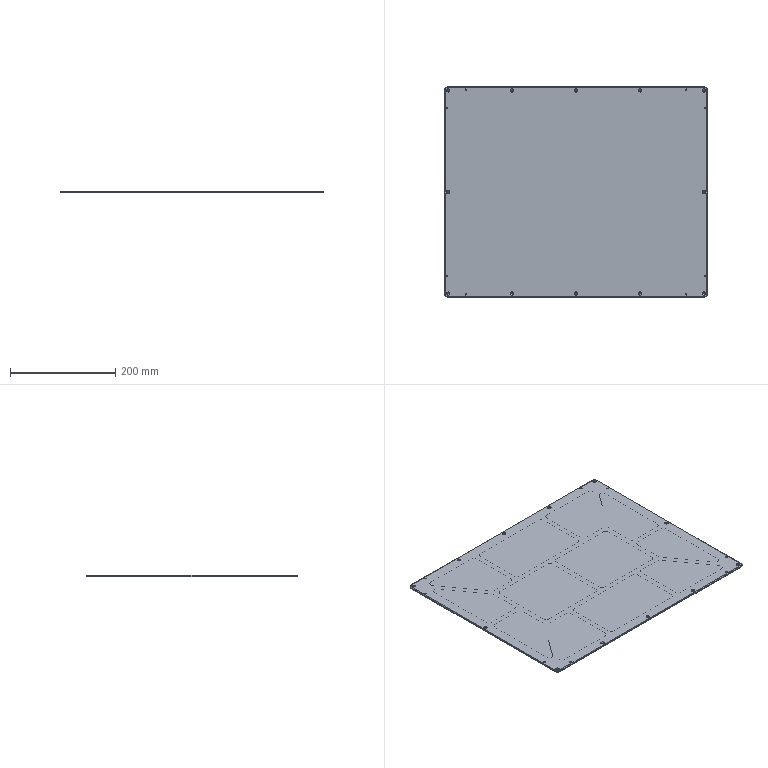NC program | Mastercam | posted with a generic post | part box 500 x 400 x 3 mm
Lines 215 to 2041 of 11256:
(8 BNOS |TOOL - 18|DIA. OFF. - 18|LEN. - 18|TOOL DIA. - 8.)
N508 T18 M6
N510 G0 G54 G90 X0. Y202.06 C0. B0. S7000 M3
N512 G43 H18 Z30.5
N514 Z19.999
N516 Z9.999
N518 G1 Z-.001 F600.
N520 X245. F4000.
N522 X245.315 Y202.053
N524 X245.958 Y201.995
N526 X246.613 Y201.873
N528 X247.272 Y201.685
N530 X247.761 Y201.498
N532 X248.243 Y201.271
N534 X248.711 Y201.006
N536 X249.161 Y200.703
N538 X249.59 Y200.364
N540 X249.992 Y199.992
N542 X250.364 Y199.59
N544 X250.703 Y199.161
N546 X251.006 Y198.711
N548 X251.271 Y198.243
N550 X251.498 Y197.761
N552 X251.685 Y197.272
N554 X251.788 Y196.943
N556 X251.942 Y196.285
N558 X252.032 Y195.634
N560 X252.06 Y195.
N562 Y-195.
N564 X252.053 Y-195.315
N566 X251.995 Y-195.958
N568 X251.873 Y-196.613
N570 X251.685 Y-197.272
N572 X251.498 Y-197.761
N574 X251.271 Y-198.243
N576 X251.006 Y-198.711
N578 X250.703 Y-199.161
N580 X250.364 Y-199.59
N582 X249.992 Y-199.992
N584 X249.59 Y-200.364
N586 X249.161 Y-200.703
N588 X248.711 Y-201.006
N590 X248.243 Y-201.271
N592 X247.761 Y-201.498
N594 X247.272 Y-201.685
N596 X246.943 Y-201.788
N598 X246.285 Y-201.942
N600 X245.634 Y-202.032
N602 X245. Y-202.06
N604 X-245.
N606 X-245.315 Y-202.053
N608 X-245.958 Y-201.995
N610 X-246.613 Y-201.873
N612 X-247.272 Y-201.685
N614 X-247.761 Y-201.498
N616 X-248.243 Y-201.271
N618 X-248.711 Y-201.006
N620 X-249.161 Y-200.703
N622 X-249.59 Y-200.364
N624 X-249.992 Y-199.992
N626 X-250.364 Y-199.59
N628 X-250.703 Y-199.161
N630 X-251.006 Y-198.711
N632 X-251.271 Y-198.243
N634 X-251.498 Y-197.761
N636 X-251.685 Y-197.272
N638 X-251.788 Y-196.943
N640 X-251.942 Y-196.285
N642 X-252.032 Y-195.634
N644 X-252.06 Y-195.
N646 Y195.
N648 X-252.053 Y195.315
N650 X-251.995 Y195.958
N652 X-251.873 Y196.613
N654 X-251.685 Y197.272
N656 X-251.498 Y197.761
N658 X-251.271 Y198.243
N660 X-251.006 Y198.711
N662 X-250.703 Y199.161
N664 X-250.364 Y199.59
N666 X-249.992 Y199.992
N668 X-249.59 Y200.364
N670 X-249.161 Y200.703
N672 X-248.711 Y201.006
N674 X-248.243 Y201.271
N676 X-247.761 Y201.498
N678 X-247.272 Y201.685
N680 X-246.943 Y201.788
N682 X-246.285 Y201.942
N684 X-245.634 Y202.032
N686 X-245. Y202.06
N688 X0.
N690 X245.336 Y202.079 Z-.002
N692 X245.979 Y202.018
N694 X246.634 Y201.896
N696 X247.293 Y201.706
N698 X247.782 Y201.518
N700 X248.264 Y201.291
N702 X248.732 Y201.025
N704 X249.182 Y200.722
N706 X249.611 Y200.383
N708 X250.013 Y200.01
N710 X250.386 Y199.608
N712 X250.724 Y199.179
N714 X251.028 Y198.728
N716 X251.293 Y198.26
N718 X251.521 Y197.779
N720 X251.708 Y197.289
N722 X251.811 Y196.96
N724 X251.967 Y196.302
N726 X252.057 Y195.651
N728 X252.088 Y195.017
N730 X252.13 Y-195.043 Z-.004
N732 X252.12 Y-195.358
N734 X252.058 Y-196.002
N736 X251.935 Y-196.657
N738 X251.744 Y-197.316
N740 X251.556 Y-197.806
N742 X251.328 Y-198.287
N744 X251.062 Y-198.756
N746 X250.758 Y-199.207
N748 X250.419 Y-199.636
N750 X250.047 Y-200.039
N752 X249.644 Y-200.412
N754 X249.216 Y-200.752
N756 X248.765 Y-201.056
N758 X248.297 Y-201.323
N760 X247.816 Y-201.552
N762 X247.327 Y-201.741
N764 X246.998 Y-201.846
N766 X246.34 Y-202.004
N768 X245.689 Y-202.096
N770 X245.055 Y-202.13
N772 X-245.096 Y-202.182 Z-.008
N774 X-245.411 Y-202.171
N776 X-246.055 Y-202.104
N778 X-246.711 Y-201.979 Z-.009
N780 X-247.369 Y-201.783
N782 X-247.858 Y-201.593
N784 X-248.339 Y-201.363
N786 X-248.807 Y-201.094
N788 X-249.257 Y-200.789
N790 X-249.686 Y-200.449
N792 X-250.089 Y-200.075
N794 X-250.462 Y-199.672
N796 X-250.801 Y-199.242
N798 X-251.105 Y-198.791
N800 X-251.373 Y-198.322
N802 X-251.601 Y-197.841
N804 X-251.791 Y-197.35
N806 X-251.896 Y-197.022
N808 X-252.056 Y-196.363
N810 X-252.149 Y-195.712
N812 X-252.184 Y-195.077
N814 X-252.226 Y195.103 Z-.013
N816 X-252.213 Y195.419
N818 X-252.145 Y196.063
N820 X-252.022 Y196.719
N822 X-251.827 Y197.378
N824 X-251.637 Y197.868
N826 X-251.407 Y198.349
N828 X-251.14 Y198.818
N830 X-250.835 Y199.27
N832 X-250.496 Y199.7
N834 X-250.123 Y200.104
N836 X-249.72 Y200.478
N838 X-249.291 Y200.819
N840 X-248.84 Y201.125
N842 X-248.373 Y201.394
N844 X-247.892 Y201.626
N846 X-247.403 Y201.818
N848 X-247.074 Y201.926
N850 X-246.417 Y202.089
N852 X-245.765 Y202.186
N854 X-245.13 Y202.226
N856 X0. Y202.259 Z-.017
N858 X245.021 Y202.287 Z-.021
N860 X245.674 Y202.255
N862 X246.342 Y202.162
N864 X246.68 Y202.09
N866 X247.019 Y202.001
N868 X247.357 Y201.895
N870 X247.861 Y201.702
N872 X248.355 Y201.468
N874 X248.837 Y201.195
N876 X249.3 Y200.883
N878 X249.741 Y200.534
N880 X250.154 Y200.151
N882 X250.537 Y199.737
N884 X250.885 Y199.296
N886 X251.197 Y198.833
N888 X251.47 Y198.352
N890 X251.704 Y197.857
N892 X251.897 Y197.353
N894 X252.003 Y197.015
N896 X252.092 Y196.676
N898 X252.163 Y196.338
N900 X252.257 Y195.67
N902 X252.288 Y195.017
N904 X252.331 Y-195.044 Z-.028
N906 X252.298 Y-195.697
N908 X252.203 Y-196.366
N910 X252.131 Y-196.704
N912 X252.041 Y-197.043
N914 X251.934 Y-197.381
N916 X251.74 Y-197.884
N918 X251.505 Y-198.379
N920 X251.231 Y-198.861 Z-.027
N922 X250.919 Y-199.324
N924 X250.57 Y-199.765 Z-.028
N926 X250.188 Y-200.18
N928 X249.774 Y-200.563
N930 X249.333 Y-200.912 Z-.027
N932 X248.87 Y-201.225
N934 X248.389 Y-201.5
N936 X247.895 Y-201.735 Z-.028
N938 X247.392 Y-201.93
N940 X247.054 Y-202.038
N942 X246.715 Y-202.128
N944 X246.377 Y-202.201
N946 X245.709 Y-202.297
N948 X245.056 Y-202.332
N950 X-245.098 Y-202.387 Z-.038
N952 X-245.752 Y-202.349
N954 X-246.42 Y-202.249
N956 X-246.758 Y-202.175
N958 X-247.097 Y-202.083
N960 X-247.435 Y-201.974
N962 X-247.938 Y-201.777
N964 X-248.432 Y-201.541
N966 X-248.913 Y-201.264
N968 X-249.376 Y-200.95
N970 X-249.816 Y-200.6
N972 X-250.23 Y-200.216
N974 X-250.613 Y-199.801
N976 X-250.962 Y-199.359
N978 X-251.275 Y-198.896
N980 X-251.549 Y-198.414
N982 X-251.785 Y-197.919
N984 X-251.98 Y-197.416
N986 X-252.089 Y-197.078
N988 X-252.18 Y-196.739
N990 X-252.254 Y-196.401
N992 X-252.352 Y-195.732
N994 X-252.388 Y-195.079
N996 X-252.431 Y195.106 Z-.047
N998 X-252.393 Y195.759
N1000 X-252.293 Y196.429
N1002 X-252.219 Y196.767
N1004 X-252.127 Y197.105
N1006 X-252.017 Y197.444
N1008 X-251.821 Y197.947
N1010 X-251.585 Y198.442
N1012 X-251.309 Y198.924
N1014 X-250.996 Y199.387
N1016 X-250.646 Y199.829
N1018 X-250.263 Y200.244
N1020 X-249.849 Y200.628
N1022 X-249.409 Y200.979
N1024 X-248.946 Y201.294
N1026 X-248.466 Y201.571
N1028 X-247.972 Y201.809
N1030 X-247.469 Y202.007
N1032 X-247.132 Y202.12
N1034 X-246.456 Y202.288
N1036 X-245.787 Y202.391
N1038 X-245.133 Y202.431
N1040 X0. Y202.462 Z-.054
N1042 X245.188 Y202.486 Z-.06
N1044 X245.523 Y202.47
N1046 X245.863 Y202.438
N1048 X246.207 Y202.39
N1050 X246.553 Y202.325
N1052 X247.075 Y202.197 Z-.061
N1054 X247.596 Y202.026
N1056 X248.111 Y201.814
N1058 X248.616 Y201.56
N1060 X249.105 Y201.265
N1062 X249.574 Y200.932
N1064 X250.018 Y200.561
N1066 X250.433 Y200.157
N1068 X250.815 Y199.722
N1070 X251.161 Y199.26
N1072 X251.469 Y198.777
N1074 X251.736 Y198.277
N1076 X251.962 Y197.765
N1078 X252.146 Y197.245
N1080 X252.29 Y196.723
N1082 X252.363 Y196.376
N1084 X252.419 Y196.03
N1086 X252.459 Y195.688
N1088 X252.483 Y195.35
N1090 X252.491 Y195.017
N1092 X252.531 Y-195.211 Z-.072
N1094 X252.514 Y-195.546
N1096 X252.481 Y-195.887
N1098 X252.432 Y-196.231
N1100 X252.366 Y-196.577
N1102 X252.237 Y-197.099 Z-.073
N1104 X252.065 Y-197.62
N1106 X251.852 Y-198.136
N1108 X251.598 Y-198.64
N1110 X251.303 Y-199.13
N1112 X250.97 Y-199.6
N1114 X250.599 Y-200.044
N1116 X250.195 Y-200.46
N1118 X249.759 Y-200.843
N1120 X249.298 Y-201.19
N1122 X248.815 Y-201.498
N1124 X248.316 Y-201.767
N1126 X247.803 Y-201.995
N1128 X247.284 Y-202.181
N1130 X246.762 Y-202.326
N1132 X246.415 Y-202.402
N1134 X246.07 Y-202.459
N1136 X245.727 Y-202.501
N1138 X245.223 Y-202.531
N1140 X-245.099 Y-202.591 Z-.089
N1142 X-245.601 Y-202.566
N1144 X-245.942 Y-202.531
N1146 X-246.286 Y-202.48
N1148 X-246.632 Y-202.412
N1150 X-247.153 Y-202.279
N1152 X-247.674 Y-202.104
N1154 X-248.189 Y-201.889
N1156 X-248.693 Y-201.632
N1158 X-249.182 Y-201.336
N1160 X-249.651 Y-201. Z-.09
N1162 X-250.096 Y-200.629
N1164 X-250.511 Y-200.223
N1166 X-250.894 Y-199.787
N1168 X-251.24 Y-199.325
N1170 X-251.549 Y-198.841
N1172 X-251.818 Y-198.341
N1174 X-252.046 Y-197.828
N1176 X-252.232 Y-197.309
N1178 X-252.378 Y-196.786 Z-.089
N1180 X-252.454 Y-196.439 Z-.09
N1182 X-252.513 Y-196.093
N1184 X-252.555 Y-195.751
N1186 X-252.592 Y-195.079
N1188 X-252.636 Y195.106 Z-.104
N1190 X-252.624 Y195.44
N1192 X-252.596 Y195.778
N1194 X-252.553 Y196.121
N1196 X-252.494 Y196.466
N1198 X-252.418 Y196.814
N1200 X-252.323 Y197.162
N1202 X-252.149 Y197.683
N1204 X-251.934 Y198.199
N1206 X-251.678 Y198.704
N1208 X-251.382 Y199.194
N1210 X-251.048 Y199.664
N1212 X-250.677 Y200.11
N1214 X-250.272 Y200.526
N1216 X-249.836 Y200.91
N1218 X-249.375 Y201.259
N1220 X-248.893 Y201.57
N1222 X-248.393 Y201.841
N1224 X-247.881 Y202.072
N1226 X-247.362 Y202.261
N1228 X-246.841 Y202.41
N1230 X-246.494 Y202.489
N1232 X-246.148 Y202.55
N1234 X-245.806 Y202.594
N1236 X-245.134 Y202.636
N1238 X0. Y202.666 Z-.114
N1240 X245.192 Y202.689 Z-.123
N1242 X245.537 Y202.673
N1244 X245.886 Y202.64
N1246 X246.239 Y202.591
N1248 X246.595 Y202.524
N1250 X247.131 Y202.393 Z-.124
N1252 X247.666 Y202.217
N1254 X248.195 Y201.999
N1256 X248.713 Y201.738
N1258 X249.216 Y201.436
N1260 X249.698 Y201.093
N1262 X250.154 Y200.712
N1264 X250.581 Y200.297
N1266 X250.973 Y199.85
N1268 X251.328 Y199.376
N1270 X251.644 Y198.879
N1272 X251.919 Y198.366
N1274 X252.151 Y197.839
N1276 X252.34 Y197.306
N1278 X252.488 Y196.769
N1280 X252.563 Y196.412
N1282 X252.621 Y196.058
N1284 X252.662 Y195.706
N1286 X252.686 Y195.359 Z-.125
N1288 X252.695 Y195.017
N1290 X252.734 Y-195.215 Z-.141
N1292 X252.716 Y-195.56
N1294 X252.683 Y-195.909
N1296 X252.633 Y-196.262
N1298 X252.565 Y-196.618 Z-.14
N1300 X252.432 Y-197.155 Z-.141
N1302 X252.256 Y-197.69
N1304 X252.037 Y-198.219
N1306 X251.775 Y-198.738
N1308 X251.472 Y-199.24
N1310 X251.129 Y-199.722
N1312 X250.749 Y-200.179
N1314 X250.333 Y-200.606
N1316 X249.887 Y-201.
N1318 X249.413 Y-201.356
N1320 X248.917 Y-201.673
N1322 X248.404 Y-201.949
N1324 X247.878 Y-202.183
N1326 X247.344 Y-202.374
N1328 X246.808 Y-202.524
N1330 X246.451 Y-202.602
N1332 X246.097 Y-202.66
N1334 X245.745 Y-202.703 Z-.142
N1336 X245.398 Y-202.729
N1338 X245.056 Y-202.739
N1340 X-245.098 Y-202.793 Z-.164
N1342 X-245.44 Y-202.782
N1344 X-245.788 Y-202.754
N1346 X-246.139 Y-202.71
N1348 X-246.494 Y-202.649
N1350 X-246.851 Y-202.57
N1352 X-247.209 Y-202.474
N1354 X-247.743 Y-202.295
N1356 X-248.272 Y-202.073
N1358 X-248.79 Y-201.809
N1360 X-249.292 Y-201.504
N1362 X-249.773 Y-201.16
N1364 X-250.23 Y-200.777
N1366 X-250.656 Y-200.361
N1368 X-251.049 Y-199.913
N1370 X-251.405 Y-199.438
N1372 X-251.722 Y-198.942
N1374 X-251.998 Y-198.428
N1376 X-252.232 Y-197.902
N1378 X-252.424 Y-197.368
N1380 X-252.574 Y-196.832
N1382 X-252.653 Y-196.475
N1384 X-252.713 Y-196.12
N1386 X-252.757 Y-195.768 Z-.165
N1388 X-252.784 Y-195.421
N1390 X-252.795 Y-195.078
N1392 X-252.837 Y195.105 Z-.184
N1394 X-252.825 Y195.448
N1396 X-252.798 Y195.795
N1398 X-252.754 Y196.147
N1400 X-252.693 Y196.502
N1402 X-252.614 Y196.859
N1404 X-252.517 Y197.217 Z-.183
N1406 X-252.338 Y197.752
N1408 X-252.116 Y198.281
N1410 X-251.853 Y198.8
N1412 X-251.549 Y199.303
N1414 X-251.205 Y199.785
N1416 X-250.824 Y200.242
N1418 X-250.408 Y200.67
N1420 X-249.961 Y201.065
N1422 X-249.488 Y201.423
N1424 X-248.992 Y201.742
N1426 X-248.48 Y202.021
N1428 X-247.954 Y202.257
N1430 X-247.421 Y202.452
N1432 X-246.885 Y202.606
N1434 X-246.529 Y202.688 Z-.184
N1436 X-245.998 Y202.772 Z-.183
N1438 X-245.649 Y202.81
N1440 X-245.133 Y202.838 Z-.184
N1442 X0. Y202.868 Z-.198
N1444 X245.196 Y202.89 Z-.21
N1446 X245.549 Y202.873
N1448 X245.908 Y202.84
N1450 X246.27 Y202.789
N1452 X246.818 Y202.682 Z-.211
N1454 X247.369 Y202.53
N1456 X247.917 Y202.336
N1458 X248.457 Y202.097
N1460 X248.984 Y201.815
N1462 X249.493 Y201.491
N1464 X249.979 Y201.126
N1466 X250.438 Y200.723
N1468 X250.865 Y200.286
N1470 X251.255 Y199.817
N1472 X251.606 Y199.322
N1474 X251.917 Y198.806
N1476 X252.184 Y198.274
N1478 X252.408 Y197.731
N1480 X252.587 Y197.182
N1482 X252.724 Y196.631
N1484 X252.82 Y196.085
N1486 X252.862 Y195.724
N1488 X252.887 Y195.368
N1490 X252.895 Y195.017 Z-.212
N1492 X252.933 Y-195.218 Z-.233
N1494 X252.915 Y-195.572
N1496 X252.881 Y-195.931 Z-.232
N1498 X252.83 Y-196.293
N1500 X252.721 Y-196.841 Z-.233
N1502 X252.569 Y-197.392 Z-.234
N1504 X252.374 Y-197.94
N1506 X252.135 Y-198.48
N1508 X251.852 Y-199.008
N1510 X251.528 Y-199.517
N1512 X251.163 Y-200.004
N1514 X250.76 Y-200.464
N1516 X250.322 Y-200.891
N1518 X249.853 Y-201.282
N1520 X249.359 Y-201.634
N1522 X248.843 Y-201.946
N1524 X248.312 Y-202.215
N1526 X247.769 Y-202.44
N1528 X247.219 Y-202.621
N1530 X246.669 Y-202.76 Z-.233
N1532 X246.122 Y-202.858
N1534 X245.761 Y-202.902 Z-.234
N1536 X245.405 Y-202.928
N1538 X245.054 Y-202.938
N1540 X-245.095 Y-202.991 Z-.263
N1542 X-245.446 Y-202.979
N1544 X-245.803 Y-202.951
N1546 X-246.164 Y-202.906
N1548 X-246.528 Y-202.844
N1550 X-246.894 Y-202.763
N1552 X-247.444 Y-202.608
N1554 X-247.992 Y-202.41
N1556 X-248.531 Y-202.169
N1558 X-249.058 Y-201.884
N1560 X-249.567 Y-201.558
N1562 X-250.054 Y-201.192
N1564 X-250.513 Y-200.787 Z-.264
N1566 X-250.939 Y-200.349
N1568 X-251.33 Y-199.88
N1570 X-251.683 Y-199.384
N1572 X-251.994 Y-198.868
N1574 X-252.263 Y-198.336
N1576 X-252.489 Y-197.792 Z-.263
N1578 X-252.671 Y-197.243
N1580 X-252.81 Y-196.692
N1582 X-252.909 Y-196.145
N1584 X-252.954 Y-195.784
N1586 X-252.981 Y-195.427 Z-.264
N1588 X-252.992 Y-195.076
N1590 X-253.033 Y195.102 Z-.288
N1592 X-253.021 Y195.453
N1594 X-252.993 Y195.81
N1596 X-252.948 Y196.171
N1598 X-252.886 Y196.536
N1600 X-252.805 Y196.902
N1602 X-252.65 Y197.453
N1604 X-252.453 Y198.001
N1606 X-252.212 Y198.541
N1608 X-251.928 Y199.069
N1610 X-251.602 Y199.579
N1612 X-251.237 Y200.066 Z-.289
N1614 X-250.833 Y200.526
N1616 X-250.395 Y200.954
N1618 X-249.927 Y201.347 Z-.288
N1620 X-249.433 Y201.701
N1622 X-248.917 Y202.014
N1624 X-248.386 Y202.286
N1626 X-247.843 Y202.514
N1628 X-247.294 Y202.699
N1630 X-246.744 Y202.841 Z-.287
N1632 X-246.197 Y202.943
N1634 X-245.837 Y202.99 Z-.288
N1636 X-245.48 Y203.02
N1638 X-245.128 Y203.033
N1640 X0. Y203.062 Z-.305
N1642 X245.199 Y203.083 Z-.32
N1644 X245.561 Y203.066
N1646 X245.929 Y203.032
N1648 X246.3 Y202.98
N1650 X246.862 Y202.87 Z-.321
N1652 X247.426 Y202.715
N1654 X247.987 Y202.516 Z-.322
N1656 X248.541 Y202.271
N1658 X249.081 Y201.982 Z-.321
N1660 X249.603 Y201.65 Z-.322
N1662 X250.101 Y201.276
N1664 X250.571 Y200.863
N1666 X251.008 Y200.415
N1668 X251.408 Y199.935
N1670 X251.768 Y199.428
N1672 X252.086 Y198.899
N1674 X252.36 Y198.354
N1676 X252.589 Y197.797
N1678 X252.773 Y197.234
N1680 X252.913 Y196.671
N1682 X253.011 Y196.11
N1684 X253.054 Y195.74
N1686 X253.079 Y195.375
N1688 X253.088 Y195.016
N1690 X253.124 Y-195.22 Z-.348
N1692 X253.106 Y-195.583
N1694 X253.071 Y-195.95
N1696 X253.019 Y-196.322
N1698 X252.907 Y-196.884 Z-.349
N1700 X252.751 Y-197.448
N1702 X252.551 Y-198.009
N1704 X252.307 Y-198.563
N1706 X252.017 Y-199.104
N1708 X251.685 Y-199.626
N1710 X251.311 Y-200.125
N1712 X250.898 Y-200.595 Z-.35
N1714 X250.449 Y-201.033 Z-.349
N1716 X249.969 Y-201.433
N1718 X249.463 Y-201.795
N1720 X248.934 Y-202.114
N1722 X248.389 Y-202.389
N1724 X247.833 Y-202.62
N1726 X247.27 Y-202.805
N1728 X246.706 Y-202.948
N1730 X246.146 Y-203.048
N1732 X245.776 Y-203.092
N1734 X245.411 Y-203.119
N1736 X245.051 Y-203.129
N1738 X-245.09 Y-203.179 Z-.385
N1740 X-245.45 Y-203.167
N1742 X-245.815 Y-203.139
N1744 X-246.185 Y-203.093
N1746 X-246.558 Y-203.03
N1748 X-246.933 Y-202.947 Z-.384
N1750 X-247.497 Y-202.789 Z-.385
N1752 X-248.058 Y-202.586
N1754 X-248.611 Y-202.339
N1756 X-249.151 Y-202.048
N1758 X-249.673 Y-201.714
N1760 X-250.171 Y-201.338
N1762 X-250.641 Y-200.924 Z-.386
N1764 X-251.079 Y-200.475
N1766 X-251.479 Y-199.994
N1768 X-251.84 Y-199.486 Z-.385
N1770 X-252.159 Y-198.957
N1772 X-252.435 Y-198.412
N1774 X-252.666 Y-197.855
N1776 X-252.852 Y-197.292
N1778 X-252.995 Y-196.728
N1780 X-253.096 Y-196.167
N1782 X-253.141 Y-195.797
N1784 X-253.169 Y-195.432
N1786 X-253.18 Y-195.072
N1788 X-253.219 Y195.096 Z-.415
N1790 X-253.193 Y195.639 Z-.414
N1792 X-253.156 Y196.007 Z-.413
N1794 X-253.101 Y196.379
N1796 X-252.986 Y196.941 Z-.414
N1798 X-252.828 Y197.505 Z-.415
N1800 X-252.626 Y198.067
N1802 X-252.38 Y198.62
N1804 X-252.089 Y199.161
N1806 X-251.755 Y199.683
N1808 X-251.381 Y200.183 Z-.416
N1810 X-250.967 Y200.654
N1812 X-250.519 Y201.092 Z-.415
N1814 X-250.039 Y201.495
N1816 X-249.532 Y201.857
N1818 X-249.004 Y202.178
N1820 X-248.459 Y202.456
N1822 X-247.903 Y202.689
N1824 X-247.341 Y202.879 Z-.414
N1826 X-246.777 Y203.024
N1828 X-246.217 Y203.128
N1830 X-245.847 Y203.176 Z-.415
N1832 X-245.122 Y203.219
N1834 X0. Y203.245 Z-.435
N1836 X245.202 Y203.265 Z-.453
N1838 X245.572 Y203.248
N1840 X245.948 Y203.213
N1842 X246.328 Y203.16
N1844 X246.902 Y203.047 Z-.454
N1846 X247.479 Y202.888
N1848 X248.053 Y202.685
N1850 X248.619 Y202.435
N1852 X249.172 Y202.139
N1854 X249.705 Y201.8
N1856 X250.215 Y201.418 Z-.455
N1858 X250.696 Y200.995
N1860 X251.143 Y200.537
N1862 X251.552 Y200.045 Z-.454
N1864 X251.92 Y199.527 Z-.455
N1866 X252.245 Y198.986
N1868 X252.525 Y198.429
N1870 X252.76 Y197.859
N1872 X252.948 Y197.284
N1874 X253.091 Y196.707
N1876 X253.192 Y196.134
N1878 X253.235 Y195.756
N1880 X253.261 Y195.382
N1882 X253.27 Y195.015
N1884 X253.303 Y-195.221 Z-.485
N1886 X253.285 Y-195.592
N1888 X253.249 Y-195.968
N1890 X253.195 Y-196.348
N1892 X253.081 Y-196.922 Z-.486
N1894 X252.922 Y-197.499
N1896 X252.717 Y-198.074
N1898 X252.467 Y-198.64
N1900 X252.171 Y-199.192
N1902 X251.831 Y-199.726
N1904 X251.449 Y-200.237 Z-.487
N1906 X251.027 Y-200.718
N1908 X250.568 Y-201.166
N1910 X250.077 Y-201.575
N1912 X249.559 Y-201.945
N1914 X249.019 Y-202.271
N1916 X248.462 Y-202.553
N1918 X247.892 Y-202.788
N1920 X247.317 Y-202.978
N1922 X246.74 Y-203.123
N1924 X246.167 Y-203.225
N1926 X245.789 Y-203.27
N1928 X245.415 Y-203.298
N1930 X245.047 Y-203.308
N1932 X-245.083 Y-203.354 Z-.528
N1934 X-245.451 Y-203.342
N1936 X-245.825 Y-203.313
N1938 X-246.203 Y-203.267
N1940 X-246.585 Y-203.202 Z-.527
N1942 X-246.968 Y-203.117
N1944 X-247.545 Y-202.956
N1946 X-248.119 Y-202.749
N1948 X-248.684 Y-202.497
N1950 X-249.236 Y-202.199
N1952 X-249.77 Y-201.857
N1954 X-250.28 Y-201.475 Z-.529
N1956 X-250.76 Y-201.051 Z-.528
N1958 X-251.208 Y-200.591 Z-.529
N1960 X-251.617 Y-200.1 Z-.528
N1962 X-251.987 Y-199.581 Z-.529
N1964 X-252.312 Y-199.04 Z-.528
N1966 X-252.595 Y-198.482 Z-.529
N1968 X-252.831 Y-197.913
N1970 X-253.021 Y-197.337
N1972 X-253.167 Y-196.76
N1974 X-253.27 Y-196.187
N1976 X-253.316 Y-195.808
N1978 X-253.344 Y-195.435
N1980 X-253.354 Y-195.066
N1982 X-253.385 Y195.273 Z-.562
N1984 X-253.365 Y195.644
N1986 X-253.327 Y196.02 Z-.561
N1988 X-253.271 Y196.4
N1990 X-253.153 Y196.975
N1992 X-252.991 Y197.552
N1994 X-252.785 Y198.126
N1996 X-252.533 Y198.692
N1998 X-252.236 Y199.245
N2000 X-251.894 Y199.779
N2002 X-251.513 Y200.291 Z-.563
N2004 X-251.09 Y200.772 Z-.562
N2006 X-250.632 Y201.22 Z-.563
N2008 X-250.141 Y201.631 Z-.562
N2010 X-249.623 Y202.002 Z-.563
N2012 X-249.083 Y202.33
N2014 X-248.526 Y202.614
N2016 X-247.957 Y202.852
N2018 X-247.382 Y203.045
N2020 X-246.806 Y203.194
N2022 X-246.232 Y203.3
N2024 X-245.854 Y203.348
N2026 X-245.481 Y203.378
N2028 X-245.112 Y203.39
N2030 X0. Y203.414 Z-.586
N2032 X245.226 Y203.431 Z-.606
N2034 X245.623 Y203.411
N2036 X246.19 Y203.351 Z-.607
N2038 X246.766 Y203.249 Z-.608
N2040 X247.345 Y203.103
N2042 X247.922 Y202.913
N2044 X248.426 Y202.709
N2046 X248.974 Y202.441
N2048 X249.506 Y202.131
N2050 X250.019 Y201.78
N2052 X250.348 Y201.524
N2054 X250.664 Y201.252
N2056 X250.966 Y200.964
N2058 X251.294 Y200.617
N2060 X251.571 Y200.29
N2062 X251.831 Y199.95
N2064 X252.072 Y199.599
N2066 X252.295 Y199.237
N2068 X252.497 Y198.868
N2070 X252.68 Y198.492
N2072 X252.915 Y197.919
N2074 X253.105 Y197.342
N2076 X253.25 Y196.763
N2078 X253.352 Y196.187
N2080 X253.397 Y195.808
N2082 X253.425 Y195.432
N2084 X253.436 Y195.013
N2086 X253.47 Y-195.033 Z-.644
N2088 X253.458 Y-195.453
N2090 X253.429 Y-195.828
N2092 X253.383 Y-196.208
N2094 X253.28 Y-196.784
N2096 X253.134 Y-197.363
N2098 X252.943 Y-197.941
N2100 X252.738 Y-198.445
N2102 X252.47 Y-198.992
N2104 X252.16 Y-199.525
N2106 X251.809 Y-200.038
N2108 X251.553 Y-200.367
N2110 X251.281 Y-200.684 Z-.645
N2112 X250.993 Y-200.987
N2114 X250.646 Y-201.315
N2116 X250.319 Y-201.593
N2118 X249.979 Y-201.853
N2120 X249.628 Y-202.095 Z-.644
N2122 X249.267 Y-202.318
N2124 X248.897 Y-202.521 Z-.645
N2126 X248.521 Y-202.704
N2128 X247.949 Y-202.941 Z-.644
N2130 X247.371 Y-203.132
N2132 X246.793 Y-203.279
N2134 X246.217 Y-203.383
N2136 X245.837 Y-203.429
N2138 X245.462 Y-203.458
N2140 X245.042 Y-203.471 Z-.645
N2142 X-245.074 Y-203.511 Z-.691
N2144 X-245.494 Y-203.497 Z-.69
N2146 X-246.059 Y-203.444 Z-.689
N2148 X-246.249 Y-203.419 Z-.69
N2150 X-246.825 Y-203.314
N2152 X-247.404 Y-203.165 Z-.691
N2154 X-247.981 Y-202.973
N2156 X-248.485 Y-202.766
N2158 X-249.032 Y-202.496 Z-.69
N2160 X-249.564 Y-202.184 Z-.691
N2162 X-250.077 Y-201.832
N2164 X-250.405 Y-201.576
N2166 X-250.722 Y-201.303
N2168 X-251.025 Y-201.014 Z-.692
N2170 X-251.352 Y-200.667 Z-.691
N2172 X-251.63 Y-200.339
N2174 X-251.89 Y-199.998
N2176 X-252.132 Y-199.647
N2178 X-252.355 Y-199.286 Z-.692
N2180 X-252.558 Y-198.916
N2182 X-252.742 Y-198.54
N2184 X-252.978 Y-197.967 Z-.691
N2186 X-253.17 Y-197.389
N2188 X-253.317 Y-196.81
N2190 X-253.422 Y-196.235
N2192 X-253.485 Y-195.667 Z-.69
N2194 X-253.512 Y-195.059 Z-.691
N2196 X-253.544 Y195.08 Z-.729
N2198 X-253.529 Y195.5
N2200 X-253.476 Y196.065 Z-.728
N2202 X-253.451 Y196.255 Z-.729
N2204 X-253.345 Y196.831
N2206 X-253.197 Y197.41
N2208 X-253.005 Y197.988
N2210 X-252.799 Y198.492
N2212 X-252.529 Y199.039
N2214 X-252.218 Y199.572
N2216 X-251.866 Y200.085
N2218 X-251.61 Y200.414 Z-.73
N2220 X-251.338 Y200.731
N2222 X-251.05 Y201.035
N2224 X-250.703 Y201.363
N2226 X-250.376 Y201.642
N2228 X-250.036 Y201.903
N2230 X-249.685 Y202.146
N2232 X-249.324 Y202.37
N2234 X-248.955 Y202.574
N2236 X-248.579 Y202.759
N2238 X-248.007 Y202.998 Z-.729
N2240 X-247.43 Y203.192
N2242 X-246.851 Y203.342
N2244 X-246.276 Y203.449
N2246 X-245.708 Y203.514 Z-.728
N2248 X-245.101 Y203.544 Z-.73
N2250 X0. Y203.565 Z-.755
N2252 X245.205 Y203.58 Z-.777
N2254 X245.59 Y203.563
N2256 X245.98 Y203.527
N2258 X246.375 Y203.472
N2260 X246.772 Y203.398
N2262 X247.171 Y203.303
N2264 X247.571 Y203.189
N2266 X247.969 Y203.053
N2268 X248.364 Y202.896
N2270 X248.755 Y202.718
N2272 X249.139 Y202.519
N2274 X249.516 Y202.299
N2276 X249.883 Y202.058
N2278 X250.239 Y201.798
N2280 X250.582 Y201.52
N2282 X250.911 Y201.223 Z-.778
N2284 X251.225 Y200.909
N2286 X251.521 Y200.58
N2288 X251.8 Y200.237
N2290 X252.06 Y199.881 Z-.777
N2292 X252.3 Y199.514 Z-.778
N2294 X252.52 Y199.137
N2296 X252.719 Y198.753
N2298 X252.897 Y198.362
N2300 X253.054 Y197.967
N2302 X253.19 Y197.568
N2304 X253.305 Y197.169
N2306 X253.399 Y196.77
N2308 X253.473 Y196.372
N2310 X253.527 Y195.978
N2312 X253.563 Y195.587
N2314 X253.581 Y195.202
N2316 X253.61 Y-195.22 Z-.817
N2318 X253.591 Y-195.605
N2320 X253.555 Y-195.995
N2322 X253.5 Y-196.39
N2324 X253.425 Y-196.788
N2326 X253.33 Y-197.187
N2328 X253.215 Y-197.587
N2330 X253.079 Y-197.985
N2332 X252.922 Y-198.38
N2334 X252.743 Y-198.771
N2336 X252.544 Y-199.156
N2338 X252.324 Y-199.532
N2340 X252.083 Y-199.9
N2342 X251.823 Y-200.256
N2344 X251.544 Y-200.599
N2346 X251.248 Y-200.929 Z-.818
N2348 X250.934 Y-201.243
N2350 X250.605 Y-201.54 Z-.817
N2352 X250.262 Y-201.819
N2354 X249.906 Y-202.079
N2356 X249.539 Y-202.32
N2358 X249.162 Y-202.54
N2360 X248.778 Y-202.74 Z-.818
N2362 X248.387 Y-202.919
N2364 X247.992 Y-203.077
N2366 X247.594 Y-203.213
N2368 X247.195 Y-203.329
N2370 X246.795 Y-203.424 Z-.817
N2372 X246.398 Y-203.499 Z-.818
N2374 X246.003 Y-203.555
N2376 X245.613 Y-203.591
N2378 X245.227 Y-203.61
N2380 X-245.064 Y-203.649 Z-.869
N2382 X-245.446 Y-203.638
N2384 X-245.834 Y-203.609
N2386 X-246.227 Y-203.562
N2388 X-246.624 Y-203.496
N2390 X-247.022 Y-203.41
N2392 X-247.422 Y-203.304
N2394 X-247.821 Y-203.177
N2396 X-248.218 Y-203.029 Z-.87
N2398 X-248.611 Y-202.86
N2400 X-248.999 Y-202.67
N2402 X-249.379 Y-202.459
N2404 X-249.751 Y-202.228
N2406 X-250.113 Y-201.977
N2408 X-250.463 Y-201.707
N2410 X-250.8 Y-201.418
N2412 X-251.121 Y-201.112
N2414 X-251.427 Y-200.79
N2416 X-251.715 Y-200.453
N2418 X-251.985 Y-200.103
N2420 X-252.235 Y-199.741
N2422 X-252.466 Y-199.368
N2424 X-252.676 Y-198.987
N2426 X-252.866 Y-198.599
N2428 X-253.034 Y-198.206
N2430 X-253.182 Y-197.809
N2432 X-253.308 Y-197.41
N2434 X-253.413 Y-197.01
N2436 X-253.499 Y-196.611
N2438 X-253.564 Y-196.214
N2440 X-253.611 Y-195.822
N2442 X-253.639 Y-195.433
N2444 X-253.65 Y-195.051
N2446 X-253.673 Y195.26 Z-.91
N2448 X-253.653 Y195.645
N2450 X-253.615 Y196.036
N2452 X-253.558 Y196.431
N2454 X-253.482 Y196.828
N2456 X-253.386 Y197.228
N2458 X-253.269 Y197.627
N2460 X-253.132 Y198.025
N2462 X-252.974 Y198.421
N2464 X-252.795 Y198.812
N2466 X-252.595 Y199.196
N2468 X-252.374 Y199.573
N2470 X-252.133 Y199.94
N2472 X-251.873 Y200.297
N2474 X-251.594 Y200.641
N2476 X-251.297 Y200.97
N2478 X-250.983 Y201.284
N2480 X-250.654 Y201.582
N2482 X-250.311 Y201.862
N2484 X-249.955 Y202.123
N2486 X-249.588 Y202.365
N2488 X-249.212 Y202.586
N2490 X-248.827 Y202.787
N2492 X-248.437 Y202.967
N2494 X-248.042 Y203.126
N2496 X-247.644 Y203.264
N2498 X-247.245 Y203.381
N2500 X-246.846 Y203.478
N2502 X-246.448 Y203.555
N2504 X-246.054 Y203.613
N2506 X-245.663 Y203.652
N2508 X-245.278 Y203.673
N2510 X0. Y203.695 Z-.938
N2512 X245.205 Y203.708 Z-.963
N2514 X245.596 Y203.69
N2516 X245.992 Y203.653
N2518 X246.393 Y203.598
N2520 X246.797 Y203.523
N2522 X247.202 Y203.427
N2524 X247.607 Y203.31
N2526 X248.012 Y203.173
N2528 X248.413 Y203.014
N2530 X248.809 Y202.833
N2532 X249.2 Y202.631
N2534 X249.582 Y202.407
N2536 X249.955 Y202.163
N2538 X250.316 Y201.899
N2540 X250.664 Y201.616
N2542 X250.999 Y201.315
N2544 X251.317 Y200.997
N2546 X251.618 Y200.663
N2548 X251.901 Y200.314
N2550 X252.165 Y199.953
N2552 X252.409 Y199.58
N2554 X252.632 Y199.198
N2556 X252.834 Y198.807
N2558 X253.015 Y198.411
N2560 X253.174 Y198.01
N2562 X253.311 Y197.605
N2564 X253.428 Y197.2
N2566 X253.523 Y196.794
N2568 X253.599 Y196.391
N2570 X253.654 Y195.99
N2572 X253.69 Y195.594
N2574 X253.708 Y195.203 Z-.964
N2576 X253.732 Y-195.218 Z-1.005
N2578 X253.714 Y-195.609
N2580 X253.677 Y-196.005
N2582 X253.621 Y-196.406
N2584 X253.545 Y-196.809
N2586 X253.449 Y-197.215
N2588 X253.333 Y-197.621
N2590 X253.195 Y-198.025
N2592 X253.035 Y-198.426
N2594 X252.854 Y-198.823
N2596 X252.652 Y-199.213
N2598 X252.428 Y-199.596
N2600 X252.184 Y-199.969
N2602 X251.92 Y-200.33
N2604 X251.637 Y-200.679
N2606 X251.336 Y-201.013
N2608 X251.018 Y-201.332
N2610 X250.684 Y-201.633
N2612 X250.335 Y-201.917
N2614 X249.974 Y-202.181
N2616 X249.601 Y-202.425
N2618 X249.219 Y-202.649
N2620 X248.828 Y-202.852
N2622 X248.432 Y-203.033 Z-1.006
N2624 X248.031 Y-203.193
N2626 X247.627 Y-203.331
N2628 X247.221 Y-203.448
N2630 X246.816 Y-203.544
N2632 X246.412 Y-203.62
N2634 X246.011 Y-203.677
N2636 X245.615 Y-203.714
N2638 X245.224 Y-203.733
N2640 X-245.053 Y-203.765 Z-1.06
N2642 X-245.441 Y-203.754
N2644 X-245.835 Y-203.726
N2646 X-246.234 Y-203.678
N2648 X-246.636 Y-203.611
N2650 X-247.041 Y-203.525
N2652 X-247.446 Y-203.417
N2654 X-247.852 Y-203.289
N2656 X-248.255 Y-203.139
N2658 X-248.654 Y-202.968
N2660 X-249.047 Y-202.775
N2662 X-249.434 Y-202.562
N2664 X-249.812 Y-202.327
N2666 X-250.179 Y-202.072 Z-1.061
N2668 X-250.534 Y-201.798
N2670 X-250.876 Y-201.505
N2672 X-251.202 Y-201.195
N2674 X-251.512 Y-200.868
N2676 X-251.805 Y-200.526
N2678 X-252.079 Y-200.17
N2680 X-252.333 Y-199.803
N2682 X-252.567 Y-199.425
N2684 X-252.78 Y-199.038
N2686 X-252.973 Y-198.644
N2688 X-253.143 Y-198.245
N2690 X-253.292 Y-197.842
N2692 X-253.42 Y-197.436
N2694 X-253.527 Y-197.03
N2696 X-253.614 Y-196.626
N2698 X-253.68 Y-196.223
N2700 X-253.727 Y-195.824
N2702 X-253.755 Y-195.43
N2704 X-253.766 Y-195.042
N2706 X-253.784 Y195.251 Z-1.103
N2708 X-253.764 Y195.642
N2710 X-253.726 Y196.038
N2712 X-253.669 Y196.439
N2714 X-253.592 Y196.843
N2716 X-253.495 Y197.248
N2718 X-253.377 Y197.654
N2720 X-253.238 Y198.058
N2722 X-253.078 Y198.46
N2724 X-252.896 Y198.856
N2726 X-252.693 Y199.247
N2728 X-252.469 Y199.629
N2730 X-252.225 Y200.002
N2732 X-251.961 Y200.364
N2734 X-251.678 Y200.713
N2736 X-251.376 Y201.047
N2738 X-251.058 Y201.366
N2740 X-250.724 Y201.668
N2742 X-250.375 Y201.952
N2744 X-250.014 Y202.217
N2746 X-249.642 Y202.462
N2748 X-249.259 Y202.686
N2750 X-248.869 Y202.89
N2752 X-248.473 Y203.072
N2754 X-248.072 Y203.233
N2756 X-247.668 Y203.373
N2758 X-247.263 Y203.491
N2760 X-246.857 Y203.589
N2762 X-246.454 Y203.667
N2764 X-246.053 Y203.724
N2766 X-245.657 Y203.763 Z-1.104
N2768 X-245.266 Y203.784
N2770 X0. Y203.802 Z-1.132
N2772 X245.205 Y203.812 Z-1.158
N2774 X245.601 Y203.794
N2776 X246.002 Y203.757
N2778 X246.408 Y203.701
N2780 X246.816 Y203.625
N2782 X247.226 Y203.528
N2784 X247.637 Y203.411
N2786 X248.046 Y203.271
N2788 X248.452 Y203.11
N2790 X248.854 Y202.927
N2792 X249.249 Y202.723
N2794 X249.636 Y202.497
N2796 X250.013 Y202.25
N2798 X250.379 Y201.983
N2800 X250.732 Y201.696
N2802 X251.07 Y201.391 Z-1.159
N2804 X251.392 Y201.069
N2806 X251.697 Y200.731
N2808 X251.984 Y200.378
N2810 X252.251 Y200.012
N2812 X252.498 Y199.635
N2814 X252.724 Y199.248
N2816 X252.928 Y198.852
N2818 X253.111 Y198.451
N2820 X253.272 Y198.045
N2822 X253.411 Y197.635
N2824 X253.529 Y197.225
N2826 X253.626 Y196.815
N2828 X253.702 Y196.406
N2830 X253.758 Y196.
N2832 X253.794 Y195.599
N2834 X253.812 Y195.204
N2836 X253.832 Y-195.215 Z-1.203
N2838 X253.813 Y-195.611
N2840 X253.776 Y-196.012
N2842 X253.72 Y-196.418 Z-1.202
N2844 X253.643 Y-196.826
N2846 X253.546 Y-197.237
N2848 X253.428 Y-197.647 Z-1.203
N2850 X253.289 Y-198.057
N2852 X253.127 Y-198.463
N2854 X252.944 Y-198.865
N2856 X252.739 Y-199.26
N2858 X252.513 Y-199.647
N2860 X252.266 Y-200.024
N2862 X251.999 Y-200.39
N2864 X251.712 Y-200.743
N2866 X251.408 Y-201.082
N2868 X251.085 Y-201.404
N2870 X250.747 Y-201.709
N2872 X250.394 Y-201.996
N2874 X250.028 Y-202.264
N2876 X249.651 Y-202.511
N2878 X249.264 Y-202.737
N2880 X248.869 Y-202.942
N2882 X248.467 Y-203.125
N2884 X248.061 Y-203.287
N2886 X247.652 Y-203.427
N2888 X247.241 Y-203.545
N2890 X246.831 Y-203.642
N2892 X246.422 Y-203.719
N2894 X246.017 Y-203.776
N2896 X245.616 Y-203.813
N2898 X245.22 Y-203.832
N2900 X-245.041 Y-203.858 Z-1.259
N2902 X-245.434 Y-203.847
N2904 X-245.833 Y-203.819
N2906 X-246.236 Y-203.771
N2908 X-246.644 Y-203.704
N2910 X-247.054 Y-203.616
N2912 X-247.464 Y-203.508
N2914 X-247.874 Y-203.379 Z-1.26
N2916 X-248.282 Y-203.227
N2918 X-248.686 Y-203.054
N2920 X-249.085 Y-202.86
N2922 X-249.476 Y-202.644
N2924 X-249.859 Y-202.406
N2926 X-250.231 Y-202.149
N2928 X-250.59 Y-201.871
N2930 X-250.936 Y-201.575
N2932 X-251.267 Y-201.261
N2934 X-251.58 Y-200.93
N2936 X-251.877 Y-200.584
N2938 X-252.154 Y-200.224
N2940 X-252.411 Y-199.852
N2942 X-252.648 Y-199.469
N2944 X-252.864 Y-199.078
N2946 X-253.058 Y-198.679
N2948 X-253.231 Y-198.275
N2950 X-253.381 Y-197.867
N2952 X-253.511 Y-197.456
N2954 X-253.619 Y-197.046
N2956 X-253.706 Y-196.636
N2958 X-253.773 Y-196.228
N2960 X-253.82 Y-195.825
N2962 X-253.848 Y-195.426
N2964 X-253.858 Y-195.033
N2966 X-253.872 Y195.241 Z-1.304
N2968 X-253.852 Y195.637
N2970 X-253.814 Y196.038
N2972 X-253.757 Y196.444
N2974 X-253.679 Y196.852
N2976 X-253.582 Y197.263
N2978 X-253.463 Y197.673
N2980 X-253.322 Y198.083
N2982 X-253.16 Y198.489
N2984 X-252.977 Y198.89
N2986 X-252.772 Y199.286
N2988 X-252.545 Y199.673
N2990 X-252.298 Y200.05
N2992 X-252.03 Y200.416
N2994 X-251.744 Y200.77
N2996 X-251.439 Y201.108
N2998 X-251.116 Y201.431
N3000 X-250.778 Y201.736
N3002 X-250.425 Y202.024
N3004 X-250.06 Y202.291
N3006 X-249.683 Y202.539
N3008 X-249.296 Y202.766
N3010 X-248.901 Y202.972
N3012 X-248.499 Y203.156
N3014 X-248.093 Y203.319
N3016 X-247.684 Y203.459
N3018 X-247.274 Y203.579
N3020 X-246.864 Y203.677
N3022 X-246.455 Y203.755
N3024 X-246.049 Y203.813
N3026 X-245.648 Y203.851
N3028 X-245.252 Y203.872 Z-1.305
N3030 X0. Y203.886 Z-1.334
N3032 X245.205 Y203.893 Z-1.36
N3034 X245.604 Y203.874
N3036 X246.009 Y203.838
N3038 X246.418 Y203.781
N3040 X246.831 Y203.704
N3042 X247.245 Y203.607
N3044 X247.66 Y203.488
N3046 X248.073 Y203.347
N3048 X248.483 Y203.185
N3050 X248.888 Y203. Z-1.361
N3052 X249.287 Y202.794 Z-1.36
N3054 X249.678 Y202.566
N3056 X250.059 Y202.317
N3058 X250.428 Y202.047
N3060 X250.784 Y201.758 Z-1.361
N3062 X251.125 Y201.45
N3064 X251.451 Y201.125
N3066 X251.759 Y200.783
N3068 X252.048 Y200.427
N3070 X252.317 Y200.058
N3072 X252.566 Y199.677
N3074 X252.794 Y199.286
N3076 X253.001 Y198.887
N3078 X253.185 Y198.482
N3080 X253.348 Y198.071
N3082 X253.489 Y197.658
N3084 X253.607 Y197.244
N3086 X253.705 Y196.83
N3088 X253.782 Y196.417
N3090 X253.838 Y196.008
N3092 X253.875 Y195.603
N3094 X253.893 Y195.203
N3096 X253.907 Y-195.211 Z-1.405
N3098 X253.889 Y-195.611
N3100 X253.851 Y-196.016
N3102 X253.795 Y-196.426
N3104 X253.718 Y-196.838
N3106 X253.62 Y-197.253
N3108 X253.501 Y-197.667
N3110 X253.36 Y-198.08
N3112 X253.197 Y-198.49
N3114 X253.013 Y-198.896
N3116 X252.806 Y-199.295
N3118 X252.578 Y-199.686
N3120 X252.329 Y-200.067
N3122 X252.059 Y-200.436
N3124 X251.77 Y-200.792
N3126 X251.462 Y-201.134 Z-1.406
N3128 X251.137 Y-201.459
N3130 X250.795 Y-201.767
N3132 X250.439 Y-202.057
N3134 X250.07 Y-202.327
N3136 X249.689 Y-202.576
N3138 X249.298 Y-202.804
N3140 X248.899 Y-203.011
N3142 X248.494 Y-203.196
N3144 X248.084 Y-203.359
N3146 X247.67 Y-203.5
N3148 X247.256 Y-203.619
N3150 X246.842 Y-203.717
N3152 X246.429 Y-203.794
N3154 X246.02 Y-203.851
N3156 X245.615 Y-203.889
N3158 X245.215 Y-203.907
N3160 X-245.03 Y-203.926 Z-1.463
N3162 X-245.426 Y-203.916
N3164 X-245.829 Y-203.888
N3166 X-246.236 Y-203.84
N3168 X-246.647 Y-203.773
N3170 X-247.061 Y-203.685
N3172 X-247.476 Y-203.576
N3174 X-247.89 Y-203.446
N3176 X-248.302 Y-203.294
N3178 X-248.709 Y-203.119
N3180 X-249.112 Y-202.923
N3182 X-249.507 Y-202.705
N3184 X-249.893 Y-202.466
N3186 X-250.268 Y-202.206
N3188 X-250.631 Y-201.926
N3190 X-250.981 Y-201.627
N3192 X-251.314 Y-201.31
N3194 X-251.631 Y-200.976
N3196 X-251.93 Y-200.627
N3198 X-252.21 Y-200.264
N3200 X-252.469 Y-199.888
N3202 X-252.708 Y-199.502
N3204 X-252.926 Y-199.107
N3206 X-253.122 Y-198.704 Z-1.464
N3208 X-253.296 Y-198.296
N3210 X-253.448 Y-197.884
N3212 X-253.578 Y-197.47 Z-1.463
N3214 X-253.687 Y-197.055
N3216 X-253.774 Y-196.641
N3218 X-253.842 Y-196.23 Z-1.464
N3220 X-253.889 Y-195.823
N3222 X-253.917 Y-195.42
N3224 X-253.927 Y-195.024
N3226 X-253.936 Y195.23 Z-1.508
N3228 X-253.916 Y195.63
N3230 X-253.878 Y196.035
N3232 X-253.821 Y196.444
N3234 X-253.744 Y196.857
N3236 X-253.645 Y197.271
N3238 X-253.526 Y197.686
N3240 X-253.384 Y198.099
N3242 X-253.221 Y198.509
N3244 X-253.036 Y198.914
N3246 X-252.829 Y199.313
N3248 X-252.601 Y199.704
N3250 X-252.351 Y200.085
N3252 X-252.081 Y200.455
N3254 X-251.792 Y200.811
N3256 X-251.484 Y201.153
N3258 X-251.159 Y201.478
N3260 X-250.817 Y201.787
N3262 X-250.461 Y202.076
N3264 X-250.092 Y202.346
N3266 X-249.711 Y202.596
N3268 X-249.321 Y202.825
N3270 X-248.922 Y203.032
N3272 X-248.516 Y203.218
N3274 X-248.107 Y203.381
N3276 X-247.694 Y203.523
N3278 X-247.279 Y203.643
N3280 X-246.865 Y203.742
N3282 X-246.452 Y203.82
N3284 X-246.043 Y203.878 Z-1.509
N3286 X-245.638 Y203.916
N3288 X-245.238 Y203.936
N3290 X0. Y203.946 Z-1.538
N3292 X245.203 Y203.95 Z-1.565
N3294 X245.606 Y203.932
N3296 X246.013 Y203.895
N3298 X246.425 Y203.838
N3300 X246.841 Y203.761
N3302 X247.258 Y203.663
N3304 X247.675 Y203.543
N3306 X248.091 Y203.402
N3308 X248.51 Y203.235
N3310 X248.93 Y203.043
N3312 X249.342 Y202.828
N3314 X249.746 Y202.59
N3316 X250.129 Y202.337
N3318 X250.489 Y202.072
N3320 X250.836 Y201.788
N3322 X251.169 Y201.487
N3324 X251.492 Y201.164
N3326 X251.802 Y200.82
N3328 X252.093 Y200.462
N3330 X252.364 Y200.09
N3332 X252.615 Y199.706
N3334 X252.845 Y199.313
N3336 X253.053 Y198.911
N3338 X253.238 Y198.503
N3340 X253.402 Y198.09
N3342 X253.543 Y197.674
N3344 X253.663 Y197.257
N3346 X253.761 Y196.84
N3348 X253.838 Y196.425
N3350 X253.895 Y196.013
N3352 X253.932 Y195.605
N3354 X253.95 Y195.203 Z-1.566
N3356 X253.959 Y-195.208 Z-1.61
N3358 X253.941 Y-195.61
N3360 X253.904 Y-196.018
N3362 X253.847 Y-196.43
N3364 X253.769 Y-196.845
N3366 X253.671 Y-197.263
N3368 X253.551 Y-197.68
N3370 X253.41 Y-198.096
N3372 X253.244 Y-198.515
N3374 X253.052 Y-198.935
N3376 X252.836 Y-199.348
N3378 X252.598 Y-199.752
N3380 X252.345 Y-200.134
N3382 X252.08 Y-200.494
N3384 X251.796 Y-200.842
N3386 X251.495 Y-201.175
N3388 X251.172 Y-201.498
N3390 X250.828 Y-201.808
N3392 X250.469 Y-202.099
N3394 X250.097 Y-202.371
N3396 X249.714 Y-202.622
N3398 X249.321 Y-202.851
N3400 X248.919 Y-203.059
N3402 X248.511 Y-203.245
N3404 X248.098 Y-203.409
N3406 X247.682 Y-203.551
N3408 X247.265 Y-203.671
N3410 X246.848 Y-203.769
N3412 X246.432 Y-203.846
N3414 X246.02 Y-203.903
N3416 X245.612 Y-203.941
N3418 X245.21 Y-203.959
N3420 X-245.018 Y-203.972 Z-1.667
N3422 X-245.417 Y-203.962
N3424 X-245.823 Y-203.934
N3426 X-246.233 Y-203.887
N3428 X-246.647 Y-203.82
N3430 X-247.063 Y-203.732
N3432 X-247.481 Y-203.622
N3434 X-247.898 Y-203.491
N3436 X-248.312 Y-203.338
N3438 X-248.735 Y-203.158
N3440 X-249.152 Y-202.954
N3442 X-249.56 Y-202.727
N3444 X-249.959 Y-202.477
N3446 X-250.325 Y-202.221
N3448 X-250.679 Y-201.946
N3450 X-251.02 Y-201.653
N3452 X-251.346 Y-201.343
N3454 X-251.665 Y-201.007
N3456 X-251.965 Y-200.655
N3458 X-252.247 Y-200.29
N3460 X-252.508 Y-199.912
N3462 X-252.749 Y-199.523
N3464 X-252.968 Y-199.125
N3466 X-253.165 Y-198.72
N3468 X-253.34 Y-198.309
N3470 X-253.493 Y-197.894
N3472 X-253.623 Y-197.477
N3474 X-253.732 Y-197.06
N3476 X-253.82 Y-196.643
N3478 X-253.888 Y-196.229
N3480 X-253.935 Y-195.819
N3482 X-253.963 Y-195.414
N3484 X-253.972 Y-195.015 Z-1.668
N3486 X-253.976 Y195.219 Z-1.712
N3488 X-253.958 Y195.621
N3490 X-253.92 Y196.029
N3492 X-253.863 Y196.442
N3494 X-253.785 Y196.857
N3496 X-253.686 Y197.274
N3498 X-253.566 Y197.691
N3500 X-253.424 Y198.107
N3502 X-253.26 Y198.52
N3504 X-253.074 Y198.928
N3506 X-252.866 Y199.33
N3508 X-252.636 Y199.723
N3510 X-252.385 Y200.107
N3512 X-252.114 Y200.479
N3514 X-251.823 Y200.838
N3516 X-251.513 Y201.181
N3518 X-251.19 Y201.505
N3520 X-250.857 Y201.806
N3522 X-250.509 Y202.09
N3524 X-250.15 Y202.356
N3526 X-249.767 Y202.609
N3528 X-249.363 Y202.848
N3530 X-248.95 Y203.063
N3532 X-248.531 Y203.256
N3534 X-248.112 Y203.423
N3536 X-247.696 Y203.565
N3538 X-247.279 Y203.685
N3540 X-246.862 Y203.784
N3542 X-246.447 Y203.862
N3544 X-246.034 Y203.919
N3546 X-245.627 Y203.957
N3548 X-245.224 Y203.976
N3550 X0. Y203.983 Z-1.741
N3552 X245.202 Y203.984 Z-1.768
N3554 X245.606 Y203.966
N3556 X246.015 Y203.929
N3558 X246.429 Y203.872
N3560 X246.846 Y203.795
N3562 X247.265 Y203.696
N3564 X247.684 Y203.576
N3566 X248.102 Y203.434
N3568 X248.523 Y203.267
N3570 X248.946 Y203.074
N3572 X249.362 Y202.857
N3574 X249.769 Y202.617
N3576 X250.153 Y202.362
N3578 X250.513 Y202.097
N3580 X250.86 Y201.813
N3582 X251.193 Y201.511
N3584 X251.517 Y201.188
N3586 X251.828 Y200.843
N3588 X252.12 Y200.483
N3590 X252.393 Y200.109
N3592 X252.645 Y199.724
N3594 X252.875 Y199.329
N3596 X253.084 Y198.926
N3598 X253.27 Y198.516
N3600 X253.434 Y198.101
N3602 X253.576 Y197.684
N3604 X253.697 Y197.265
N3606 X253.795 Y196.846
N3608 X253.872 Y196.429
N3610 X253.929 Y196.015
N3612 X253.966 Y195.605
N3614 X253.984 Y195.202
N3616 X253.989 Y-195.204 Z-1.812
N3618 X253.971 Y-195.608
N3620 X253.933 Y-196.017
N3622 X253.876 Y-196.431
N3624 X253.799 Y-196.848
N3626 X253.701 Y-197.267
N3628 X253.58 Y-197.686
N3630 X253.438 Y-198.104
N3632 X253.271 Y-198.525
N3634 X253.078 Y-198.948
N3636 X252.861 Y-199.364
N3638 X252.621 Y-199.771
N3640 X252.366 Y-200.155
N3642 X252.101 Y-200.515
N3644 X251.817 Y-200.863
N3646 X251.515 Y-201.196
N3648 X251.191 Y-201.52
N3650 X250.846 Y-201.831
N3652 X250.486 Y-202.123
N3654 X250.113 Y-202.396
N3656 X249.728 Y-202.648
N3658 X249.333 Y-202.878
N3660 X248.929 Y-203.087
N3662 X248.519 Y-203.274
N3664 X248.105 Y-203.438
N3666 X247.687 Y-203.58
N3668 X247.268 Y-203.7
N3670 X246.849 Y-203.799
N3672 X246.432 Y-203.876
N3674 X246.018 Y-203.933
N3676 X245.609 Y-203.971
N3678 X245.205 Y-203.989 Z-1.813
N3680 X-245.008 Y-203.996 Z-1.867
N3682 X-245.408 Y-203.986
N3684 X-245.815 Y-203.959
N3686 X-246.227 Y-203.911
N3688 X-246.643 Y-203.844
N3690 X-247.061 Y-203.756
N3692 X-247.48 Y-203.647
N3694 X-247.899 Y-203.516
N3696 X-248.315 Y-203.362
N3698 X-248.741 Y-203.181
N3700 X-249.161 Y-202.975
N3702 X-249.573 Y-202.746 Z-1.868
N3704 X-249.776 Y-202.623 Z-1.867
N3706 X-250.159 Y-202.369
N3708 X-250.519 Y-202.103
N3710 X-250.867 Y-201.819
N3712 X-251.2 Y-201.517
N3714 X-251.524 Y-201.194
N3716 X-251.835 Y-200.848 Z-1.868
N3718 X-252.127 Y-200.488
N3720 X-252.4 Y-200.115
N3722 X-252.652 Y-199.73
N3724 X-252.882 Y-199.335
N3726 X-253.091 Y-198.931
N3728 X-253.278 Y-198.521
N3730 X-253.442 Y-198.107
N3732 X-253.584 Y-197.689
N3734 X-253.705 Y-197.27
N3736 X-253.803 Y-196.851
N3738 X-253.881 Y-196.434
N3740 X-253.938 Y-196.02
N3742 X-253.975 Y-195.611
N3744 X-253.993 Y-195.207
N3746 X-253.996 Y195.209 Z-1.911
N3748 X-253.977 Y195.613
N3750 X-253.94 Y196.022
N3752 X-253.883 Y196.436
N3754 X-253.805 Y196.853
N3756 X-253.707 Y197.272
N3758 X-253.586 Y197.691
N3760 X-253.444 Y198.109
N3762 X-253.28 Y198.523
N3764 X-253.093 Y198.933 Z-1.912
N3766 X-252.884 Y199.336
N3768 X-252.654 Y199.731
N3770 X-252.402 Y200.116
N3772 X-252.129 Y200.49
N3774 X-251.837 Y200.85
N3776 X-251.526 Y201.195
N3778 X-251.202 Y201.519
N3780 X-250.869 Y201.821
N3782 X-250.522 Y202.105
N3784 X-250.162 Y202.37
N3786 X-249.778 Y202.625
N3788 X-249.575 Y202.748
N3790 X-249.163 Y202.977
N3792 X-248.744 Y203.182
N3794 X-248.318 Y203.364
N3796 X-247.901 Y203.517
N3798 X-247.483 Y203.649
N3800 X-247.064 Y203.758
N3802 X-246.646 Y203.846
N3804 X-246.23 Y203.914
N3806 X-245.818 Y203.961
N3808 X-245.411 Y203.989
N3810 X-245.011 Y203.998
N3812 X0. Y203.999 Z-1.94
N3814 X245.2 Y203.997
N3816 X245.604 Y203.979
N3818 X246.014 Y203.942
N3820 X246.429 Y203.885
N3822 X246.847 Y203.808
N3824 X247.266 Y203.709
N3826 X247.686 Y203.589
N3828 X248.104 Y203.447
N3830 X248.527 Y203.279
N3832 X248.951 Y203.085
N3834 X249.369 Y202.868
N3836 X249.777 Y202.627
N3838 X249.977 Y202.497
N3840 X250.343 Y202.241
N3842 X250.697 Y201.966
N3844 X251.037 Y201.673
N3846 X251.363 Y201.363
N3848 X251.682 Y201.028
N3850 X251.982 Y200.677
N3852 X252.264 Y200.313
N3854 X252.525 Y199.935
N3856 X252.769 Y199.542
N3858 X252.991 Y199.139
N3860 X253.19 Y198.729
N3862 X253.367 Y198.313
N3864 X253.521 Y197.895
N3866 X253.652 Y197.476
N3868 X253.761 Y197.056
N3870 X253.849 Y196.638
N3872 X253.916 Y196.221
N3874 X253.963 Y195.809
N3876 X253.99 Y195.401
N3878 X253.999 Y195.
N3880 X253.997 Y-195.2
N3882 X253.979 Y-195.604
N3884 X253.942 Y-196.014
N3886 X253.885 Y-196.429
N3888 X253.808 Y-196.847
N3890 X253.709 Y-197.266
N3892 X253.589 Y-197.686
N3894 X253.447 Y-198.104
N3896 X253.279 Y-198.527
N3898 X253.085 Y-198.951
N3900 X252.868 Y-199.369
N3902 X252.627 Y-199.777
N3904 X252.497 Y-199.977
N3906 X252.241 Y-200.343
N3908 X251.966 Y-200.697
N3910 X251.673 Y-201.037
N3912 X251.363 Y-201.363
N3914 X251.028 Y-201.682
N3916 X250.677 Y-201.982
N3918 X250.313 Y-202.264
N3920 X249.935 Y-202.525
N3922 X249.542 Y-202.769
N3924 X249.139 Y-202.991
N3926 X248.729 Y-203.19
N3928 X248.313 Y-203.367
N3930 X247.895 Y-203.521
N3932 X247.476 Y-203.652
N3934 X247.056 Y-203.761
N3936 X246.638 Y-203.849
N3938 X246.221 Y-203.916
N3940 X245.809 Y-203.963
N3942 X245.401 Y-203.99
N3944 X245. Y-203.999
N3946 X-245.2 Y-203.997
N3948 X-245.604 Y-203.979
N3950 X-246.014 Y-203.942
N3952 X-246.429 Y-203.885
N3954 X-246.847 Y-203.808
N3956 X-247.266 Y-203.709
N3958 X-247.686 Y-203.589
N3960 X-248.104 Y-203.447
N3962 X-248.527 Y-203.279
N3964 X-248.951 Y-203.085
N3966 X-249.369 Y-202.868
N3968 X-249.777 Y-202.627
N3970 X-249.977 Y-202.497
N3972 X-250.343 Y-202.241
N3974 X-250.697 Y-201.966
N3976 X-251.037 Y-201.673
N3978 X-251.363 Y-201.363
N3980 X-251.682 Y-201.028
N3982 X-251.982 Y-200.677
N3984 X-252.264 Y-200.313
N3986 X-252.525 Y-199.935
N3988 X-252.769 Y-199.542
N3990 X-252.991 Y-199.139
N3992 X-253.19 Y-198.729
N3994 X-253.367 Y-198.313
N3996 X-253.521 Y-197.895
N3998 X-253.652 Y-197.476
N4000 X-253.761 Y-197.056
N4002 X-253.849 Y-196.638
N4004 X-253.916 Y-196.221
N4006 X-253.963 Y-195.809
N4008 X-253.99 Y-195.401
N4010 X-253.999 Y-195.
N4012 X-253.997 Y195.2
N4014 X-253.979 Y195.604
N4016 X-253.942 Y196.014
N4018 X-253.885 Y196.429
N4020 X-253.808 Y196.847
N4022 X-253.709 Y197.266
N4024 X-253.589 Y197.686
N4026 X-253.447 Y198.104
N4028 X-253.282 Y198.521
N4030 X-253.093 Y198.935
N4032 X-252.883 Y199.342
N4034 X-252.65 Y199.74
N4036 X-252.397 Y200.125
N4038 X-252.125 Y200.497
N4040 X-251.834 Y200.855
N4042 X-251.525 Y201.198
N4044 X-251.202 Y201.52
N4046 X-250.869 Y201.822
N4048 X-250.521 Y202.106
N4050 X-250.161 Y202.372
N4052 X-249.777 Y202.627
N4054 X-249.369 Y202.868
N4056 X-249.161 Y202.979
N4058 X-248.74 Y203.185
N4060 X-248.313 Y203.367
N4062 X-247.895 Y203.521
N4064 X-247.476 Y203.652
N4066 X-247.056 Y203.761
N4068 X-246.638 Y203.849
N4070 X-246.221 Y203.916
N4072 X-245.809 Y203.963
N4074 X-245.401 Y203.99
N4076 X-245. Y203.999
N4078 X0.
N4080 G0 Z8.06
N4082 Z18.06
N4084 Z30.5
N4086 M5
N4088 G0 G28 G91 Z0.
N4090 G28
N4092 M01
N4094 G0 G17 G40 G80 G90 G94 G98
N4096 G0 G28 G91 Z0.
(4 CHM |TOOL - 5|DIA. OFF. - 5|LEN. - 5|TOOL DIA. - 4.)
N4098 T5 M6
N4100 G0 G54 G90 X243.5 Y0. C0. B0. S6000 M3
N4102 G43 H5 Z50.
N4104 G81 G98 Z-.7 R1. F200.
N4106 X245. Y-160.
N4108 X243.5 Y-193.5
N4110 X210. Y-195.
N4112 X122. Y-193.5
N4114 X0.
N4116 X-122.
N4118 X-210. Y-195.
N4120 X-243.5 Y-193.5
N4122 X-245. Y-160.
N4124 X-243.5 Y0.
N4126 X-245. Y160.
N4128 X-243.5 Y193.5
N4130 X-210. Y195.
N4132 X-122. Y193.5
N4134 X0.
N4136 X122.
N4138 X210. Y195.
N4140 X243.5 Y193.5
N4142 X245. Y160.
N4144 G80
N4146 M5
N4148 G0 G28 G91 Z0.
N4150 G28
N4152 M01
N4154 G0 G17 G40 G80 G90 G94 G98
N4156 G0 G28 G91 Z0.